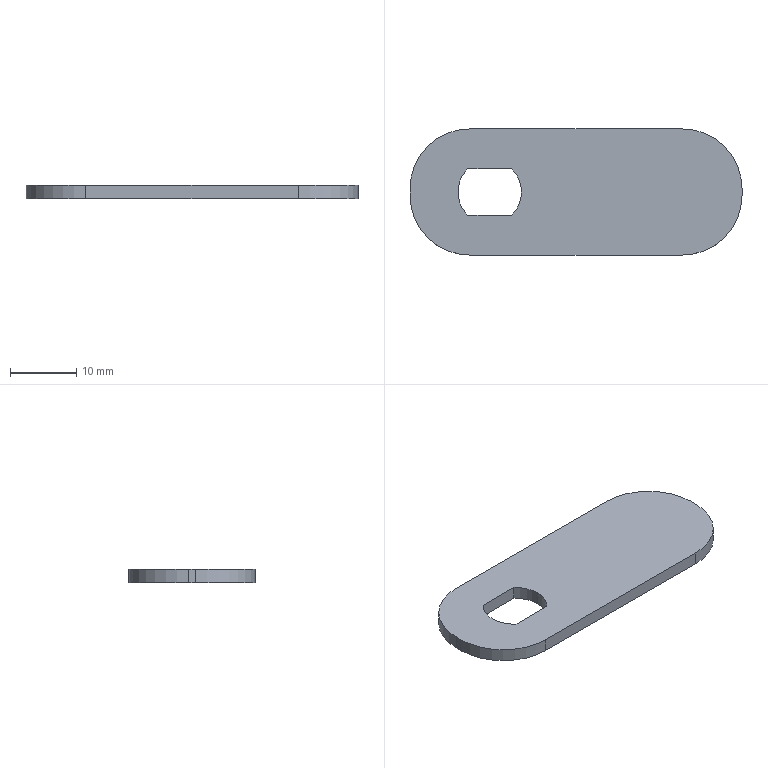Part | SolidWorks | features Fillet 1, FlatPattern 1, ICE 1, SMBaseFlange 1, SheetMetal 1 | 1 solid | 15 faces | box 50 x 19 x 2 mm | volume 1640 mm3 | plane 8 | cylinder 7 | commonest cylinder face diameters 18 x4 9.6 x3
STEP:
#1=CARTESIAN_POINT('',(-8.2,0.,-2.));
#2=VERTEX_POINT('',#1);
#3=CARTESIAN_POINT('',(-9.715,3.5,-2.));
#4=VERTEX_POINT('',#3);
#5=CARTESIAN_POINT('',(-13.,0.,-2.));
#6=DIRECTION('',(0.,0.,1.));
#7=DIRECTION('',(1.,0.,0.));
#8=AXIS2_PLACEMENT_3D('',#5,#6,#7);
#9=CIRCLE('',#8,4.8);
#10=EDGE_CURVE('',#2,#4,#9,.T.);
#11=ORIENTED_EDGE('',*,*,#10,.F.);
#12=CARTESIAN_POINT('',(-8.2,0.,0.));
#13=VERTEX_POINT('',#12);
#14=CARTESIAN_POINT('',(-8.2,0.,-10.));
#15=DIRECTION('',(0.,0.,1.));
#16=VECTOR('',#15,1000.);
#17=LINE('',#14,#16);
#18=EDGE_CURVE('',#2,#13,#17,.T.);
#19=ORIENTED_EDGE('',*,*,#18,.T.);
#20=CARTESIAN_POINT('',(-9.715,3.5,0.));
#21=VERTEX_POINT('',#20);
#22=CARTESIAN_POINT('',(-13.,0.,0.));
#23=DIRECTION('',(0.,0.,1.));
#24=DIRECTION('',(1.,0.,0.));
#25=AXIS2_PLACEMENT_3D('',#22,#23,#24);
#26=CIRCLE('',#25,4.8);
#27=EDGE_CURVE('',#13,#21,#26,.T.);
#28=ORIENTED_EDGE('',*,*,#27,.T.);
#29=CARTESIAN_POINT('',(-9.715,3.5,-10.));
#30=DIRECTION('',(0.,0.,1.));
#31=VECTOR('',#30,1000.);
#32=LINE('',#29,#31);
#33=EDGE_CURVE('',#4,#21,#32,.T.);
#34=ORIENTED_EDGE('',*,*,#33,.F.);
#35=EDGE_LOOP('',(#11,#19,#28,#34));
#36=FACE_OUTER_BOUND('',#35,.T.);
#37=CARTESIAN_POINT('',(-13.,0.,-10.));
#38=DIRECTION('',(0.,0.,1.));
#39=DIRECTION('',(1.,0.,0.));
#40=AXIS2_PLACEMENT_3D('',#37,#38,#39);
#41=CYLINDRICAL_SURFACE('',#40,4.8);
#42=ADVANCED_FACE('',(#36),#41,.F.);
#43=CARTESIAN_POINT('',(25.,-0.5,0.));
#44=VERTEX_POINT('',#43);
#45=CARTESIAN_POINT('',(25.,0.5,0.));
#46=VERTEX_POINT('',#45);
#47=CARTESIAN_POINT('',(25.,9.5,0.));
#48=DIRECTION('',(0.,1.,0.));
#49=VECTOR('',#48,1000.);
#50=LINE('',#47,#49);
#51=EDGE_CURVE('',#44,#46,#50,.T.);
#52=ORIENTED_EDGE('',*,*,#51,.F.);
#53=CARTESIAN_POINT('',(25.,-0.5,-2.));
#54=VERTEX_POINT('',#53);
#55=CARTESIAN_POINT('',(25.,-0.5,-2.));
#56=DIRECTION('',(0.,0.,-1.));
#57=VECTOR('',#56,1000.);
#58=LINE('',#55,#57);
#59=EDGE_CURVE('',#44,#54,#58,.T.);
#60=ORIENTED_EDGE('',*,*,#59,.T.);
#61=CARTESIAN_POINT('',(25.,0.5,-2.));
#62=VERTEX_POINT('',#61);
#63=CARTESIAN_POINT('',(25.,9.5,-2.));
#64=DIRECTION('',(0.,1.,0.));
#65=VECTOR('',#64,1000.);
#66=LINE('',#63,#65);
#67=EDGE_CURVE('',#54,#62,#66,.T.);
#68=ORIENTED_EDGE('',*,*,#67,.T.);
#69=CARTESIAN_POINT('',(25.,0.5,-2.));
#70=DIRECTION('',(0.,0.,1.));
#71=VECTOR('',#70,1000.);
#72=LINE('',#69,#71);
#73=EDGE_CURVE('',#62,#46,#72,.T.);
#74=ORIENTED_EDGE('',*,*,#73,.T.);
#75=EDGE_LOOP('',(#52,#60,#68,#74));
#76=FACE_OUTER_BOUND('',#75,.T.);
#77=CARTESIAN_POINT('',(25.,9.5,-2.));
#78=DIRECTION('',(1.,0.,0.));
#79=DIRECTION('',(0.,1.,0.));
#80=AXIS2_PLACEMENT_3D('',#77,#78,#79);
#81=PLANE('',#80);
#82=ADVANCED_FACE('',(#76),#81,.T.);
#83=CARTESIAN_POINT('',(-16.,-9.5,-2.));
#84=VERTEX_POINT('',#83);
#85=CARTESIAN_POINT('',(16.,-9.5,-2.));
#86=VERTEX_POINT('',#85);
#87=CARTESIAN_POINT('',(-25.,-9.5,-2.));
#88=DIRECTION('',(1.,0.,0.));
#89=VECTOR('',#88,1000.);
#90=LINE('',#87,#89);
#91=EDGE_CURVE('',#84,#86,#90,.T.);
#92=ORIENTED_EDGE('',*,*,#91,.T.);
#93=CARTESIAN_POINT('',(16.,-9.5,0.));
#94=VERTEX_POINT('',#93);
#95=CARTESIAN_POINT('',(16.,-9.5,-2.));
#96=DIRECTION('',(0.,0.,1.));
#97=VECTOR('',#96,1000.);
#98=LINE('',#95,#97);
#99=EDGE_CURVE('',#86,#94,#98,.T.);
#100=ORIENTED_EDGE('',*,*,#99,.T.);
#101=CARTESIAN_POINT('',(-16.,-9.5,0.));
#102=VERTEX_POINT('',#101);
#103=CARTESIAN_POINT('',(-25.,-9.5,0.));
#104=DIRECTION('',(1.,0.,0.));
#105=VECTOR('',#104,1000.);
#106=LINE('',#103,#105);
#107=EDGE_CURVE('',#102,#94,#106,.T.);
#108=ORIENTED_EDGE('',*,*,#107,.F.);
#109=CARTESIAN_POINT('',(-16.,-9.5,-2.));
#110=DIRECTION('',(0.,0.,-1.));
#111=VECTOR('',#110,1000.);
#112=LINE('',#109,#111);
#113=EDGE_CURVE('',#102,#84,#112,.T.);
#114=ORIENTED_EDGE('',*,*,#113,.T.);
#115=EDGE_LOOP('',(#92,#100,#108,#114));
#116=FACE_OUTER_BOUND('',#115,.T.);
#117=CARTESIAN_POINT('',(-25.,-9.5,-2.));
#118=DIRECTION('',(0.,-1.,0.));
#119=DIRECTION('',(0.,0.,-1.));
#120=AXIS2_PLACEMENT_3D('',#117,#118,#119);
#121=PLANE('',#120);
#122=ADVANCED_FACE('',(#116),#121,.T.);
#123=CARTESIAN_POINT('',(-25.,0.5,-2.));
#124=VERTEX_POINT('',#123);
#125=CARTESIAN_POINT('',(-25.,-0.5,-2.));
#126=VERTEX_POINT('',#125);
#127=CARTESIAN_POINT('',(-25.,9.5,-2.));
#128=DIRECTION('',(0.,-1.,0.));
#129=VECTOR('',#128,1000.);
#130=LINE('',#127,#129);
#131=EDGE_CURVE('',#124,#126,#130,.T.);
#132=ORIENTED_EDGE('',*,*,#131,.T.);
#133=CARTESIAN_POINT('',(-25.,-0.5,0.));
#134=VERTEX_POINT('',#133);
#135=CARTESIAN_POINT('',(-25.,-0.5,-2.));
#136=DIRECTION('',(0.,0.,1.));
#137=VECTOR('',#136,1000.);
#138=LINE('',#135,#137);
#139=EDGE_CURVE('',#126,#134,#138,.T.);
#140=ORIENTED_EDGE('',*,*,#139,.T.);
#141=CARTESIAN_POINT('',(-25.,0.5,0.));
#142=VERTEX_POINT('',#141);
#143=CARTESIAN_POINT('',(-25.,9.5,0.));
#144=DIRECTION('',(0.,-1.,0.));
#145=VECTOR('',#144,1000.);
#146=LINE('',#143,#145);
#147=EDGE_CURVE('',#142,#134,#146,.T.);
#148=ORIENTED_EDGE('',*,*,#147,.F.);
#149=CARTESIAN_POINT('',(-25.,0.5,-2.));
#150=DIRECTION('',(0.,0.,-1.));
#151=VECTOR('',#150,1000.);
#152=LINE('',#149,#151);
#153=EDGE_CURVE('',#142,#124,#152,.T.);
#154=ORIENTED_EDGE('',*,*,#153,.T.);
#155=EDGE_LOOP('',(#132,#140,#148,#154));
#156=FACE_OUTER_BOUND('',#155,.T.);
#157=CARTESIAN_POINT('',(-25.,9.5,-2.));
#158=DIRECTION('',(-1.,0.,0.));
#159=DIRECTION('',(0.,0.,1.));
#160=AXIS2_PLACEMENT_3D('',#157,#158,#159);
#161=PLANE('',#160);
#162=ADVANCED_FACE('',(#156),#161,.T.);
#163=CARTESIAN_POINT('',(16.,9.5,0.));
#164=VERTEX_POINT('',#163);
#165=CARTESIAN_POINT('',(-16.,9.5,0.));
#166=VERTEX_POINT('',#165);
#167=CARTESIAN_POINT('',(-25.,9.5,0.));
#168=DIRECTION('',(-1.,0.,0.));
#169=VECTOR('',#168,1000.);
#170=LINE('',#167,#169);
#171=EDGE_CURVE('',#164,#166,#170,.T.);
#172=ORIENTED_EDGE('',*,*,#171,.F.);
#173=CARTESIAN_POINT('',(16.,9.5,-2.));
#174=VERTEX_POINT('',#173);
#175=CARTESIAN_POINT('',(16.,9.5,-2.));
#176=DIRECTION('',(0.,0.,-1.));
#177=VECTOR('',#176,1000.);
#178=LINE('',#175,#177);
#179=EDGE_CURVE('',#164,#174,#178,.T.);
#180=ORIENTED_EDGE('',*,*,#179,.T.);
#181=CARTESIAN_POINT('',(-16.,9.5,-2.));
#182=VERTEX_POINT('',#181);
#183=CARTESIAN_POINT('',(-25.,9.5,-2.));
#184=DIRECTION('',(-1.,0.,0.));
#185=VECTOR('',#184,1000.);
#186=LINE('',#183,#185);
#187=EDGE_CURVE('',#174,#182,#186,.T.);
#188=ORIENTED_EDGE('',*,*,#187,.T.);
#189=CARTESIAN_POINT('',(-16.,9.5,-2.));
#190=DIRECTION('',(0.,0.,1.));
#191=VECTOR('',#190,1000.);
#192=LINE('',#189,#191);
#193=EDGE_CURVE('',#182,#166,#192,.T.);
#194=ORIENTED_EDGE('',*,*,#193,.T.);
#195=EDGE_LOOP('',(#172,#180,#188,#194));
#196=FACE_OUTER_BOUND('',#195,.T.);
#197=CARTESIAN_POINT('',(-25.,9.5,-2.));
#198=DIRECTION('',(0.,1.,0.));
#199=DIRECTION('',(0.,0.,1.));
#200=AXIS2_PLACEMENT_3D('',#197,#198,#199);
#201=PLANE('',#200);
#202=ADVANCED_FACE('',(#196),#201,.T.);
#203=CARTESIAN_POINT('',(-16.285,-3.5,-2.));
#204=VERTEX_POINT('',#203);
#205=CARTESIAN_POINT('',(-9.715,-3.5,-2.));
#206=VERTEX_POINT('',#205);
#207=CARTESIAN_POINT('',(0.,-3.5,-2.));
#208=DIRECTION('',(1.,0.,0.));
#209=VECTOR('',#208,1000.);
#210=LINE('',#207,#209);
#211=EDGE_CURVE('',#204,#206,#210,.T.);
#212=ORIENTED_EDGE('',*,*,#211,.T.);
#213=CARTESIAN_POINT('',(-13.,0.,-2.));
#214=DIRECTION('',(0.,0.,1.));
#215=DIRECTION('',(1.,0.,0.));
#216=AXIS2_PLACEMENT_3D('',#213,#214,#215);
#217=CIRCLE('',#216,4.8);
#218=EDGE_CURVE('',#206,#2,#217,.T.);
#219=ORIENTED_EDGE('',*,*,#218,.T.);
#220=ORIENTED_EDGE('',*,*,#10,.T.);
#221=CARTESIAN_POINT('',(-16.285,3.5,-2.));
#222=VERTEX_POINT('',#221);
#223=CARTESIAN_POINT('',(0.,3.5,-2.));
#224=DIRECTION('',(-1.,0.,0.));
#225=VECTOR('',#224,1000.);
#226=LINE('',#223,#225);
#227=EDGE_CURVE('',#4,#222,#226,.T.);
#228=ORIENTED_EDGE('',*,*,#227,.T.);
#229=CARTESIAN_POINT('',(-13.,0.,-2.));
#230=DIRECTION('',(0.,0.,1.));
#231=DIRECTION('',(1.,0.,0.));
#232=AXIS2_PLACEMENT_3D('',#229,#230,#231);
#233=CIRCLE('',#232,4.8);
#234=EDGE_CURVE('',#222,#204,#233,.T.);
#235=ORIENTED_EDGE('',*,*,#234,.T.);
#236=EDGE_LOOP('',(#212,#219,#220,#228,#235));
#237=FACE_BOUND('',#236,.T.);
#238=ORIENTED_EDGE('',*,*,#67,.F.);
#239=CARTESIAN_POINT('',(16.,-0.5,-2.));
#240=DIRECTION('',(0.,0.,-1.));
#241=DIRECTION('',(1.,0.,0.));
#242=AXIS2_PLACEMENT_3D('',#239,#240,#241);
#243=CIRCLE('',#242,9.);
#244=EDGE_CURVE('',#54,#86,#243,.T.);
#245=ORIENTED_EDGE('',*,*,#244,.T.);
#246=ORIENTED_EDGE('',*,*,#91,.F.);
#247=CARTESIAN_POINT('',(-16.,-0.5,-2.));
#248=DIRECTION('',(0.,0.,-1.));
#249=DIRECTION('',(1.,0.,0.));
#250=AXIS2_PLACEMENT_3D('',#247,#248,#249);
#251=CIRCLE('',#250,9.);
#252=EDGE_CURVE('',#84,#126,#251,.T.);
#253=ORIENTED_EDGE('',*,*,#252,.T.);
#254=ORIENTED_EDGE('',*,*,#131,.F.);
#255=CARTESIAN_POINT('',(-16.,0.5,-2.));
#256=DIRECTION('',(0.,0.,-1.));
#257=DIRECTION('',(1.,0.,0.));
#258=AXIS2_PLACEMENT_3D('',#255,#256,#257);
#259=CIRCLE('',#258,9.);
#260=EDGE_CURVE('',#124,#182,#259,.T.);
#261=ORIENTED_EDGE('',*,*,#260,.T.);
#262=ORIENTED_EDGE('',*,*,#187,.F.);
#263=CARTESIAN_POINT('',(16.,0.5,-2.));
#264=DIRECTION('',(0.,0.,-1.));
#265=DIRECTION('',(1.,0.,0.));
#266=AXIS2_PLACEMENT_3D('',#263,#264,#265);
#267=CIRCLE('',#266,9.);
#268=EDGE_CURVE('',#174,#62,#267,.T.);
#269=ORIENTED_EDGE('',*,*,#268,.T.);
#270=EDGE_LOOP('',(#238,#245,#246,#253,#254,#261,#262,#269));
#271=FACE_OUTER_BOUND('',#270,.T.);
#272=CARTESIAN_POINT('',(0.,0.,-2.));
#273=DIRECTION('',(0.,0.,1.));
#274=DIRECTION('',(1.,0.,0.));
#275=AXIS2_PLACEMENT_3D('',#272,#273,#274);
#276=PLANE('',#275);
#277=ADVANCED_FACE('',(#237,#271),#276,.F.);
#278=CARTESIAN_POINT('',(-9.715,-3.5,0.));
#279=VERTEX_POINT('',#278);
#280=CARTESIAN_POINT('',(-13.,0.,0.));
#281=DIRECTION('',(0.,0.,1.));
#282=DIRECTION('',(1.,0.,0.));
#283=AXIS2_PLACEMENT_3D('',#280,#281,#282);
#284=CIRCLE('',#283,4.8);
#285=EDGE_CURVE('',#279,#13,#284,.T.);
#286=ORIENTED_EDGE('',*,*,#285,.F.);
#287=CARTESIAN_POINT('',(-16.285,-3.5,0.));
#288=VERTEX_POINT('',#287);
#289=CARTESIAN_POINT('',(-16.285,-3.5,0.));
#290=DIRECTION('',(1.,0.,0.));
#291=VECTOR('',#290,1000.);
#292=LINE('',#289,#291);
#293=EDGE_CURVE('',#288,#279,#292,.T.);
#294=ORIENTED_EDGE('',*,*,#293,.F.);
#295=CARTESIAN_POINT('',(-16.285,3.5,0.));
#296=VERTEX_POINT('',#295);
#297=CARTESIAN_POINT('',(-13.,0.,0.));
#298=DIRECTION('',(0.,0.,1.));
#299=DIRECTION('',(1.,0.,0.));
#300=AXIS2_PLACEMENT_3D('',#297,#298,#299);
#301=CIRCLE('',#300,4.8);
#302=EDGE_CURVE('',#296,#288,#301,.T.);
#303=ORIENTED_EDGE('',*,*,#302,.F.);
#304=CARTESIAN_POINT('',(-16.285,3.5,0.));
#305=DIRECTION('',(-1.,0.,0.));
#306=VECTOR('',#305,1000.);
#307=LINE('',#304,#306);
#308=EDGE_CURVE('',#21,#296,#307,.T.);
#309=ORIENTED_EDGE('',*,*,#308,.F.);
#310=ORIENTED_EDGE('',*,*,#27,.F.);
#311=EDGE_LOOP('',(#286,#294,#303,#309,#310));
#312=FACE_BOUND('',#311,.T.);
#313=ORIENTED_EDGE('',*,*,#107,.T.);
#314=CARTESIAN_POINT('',(16.,-0.5,0.));
#315=DIRECTION('',(0.,0.,1.));
#316=DIRECTION('',(1.,0.,0.));
#317=AXIS2_PLACEMENT_3D('',#314,#315,#316);
#318=CIRCLE('',#317,9.);
#319=EDGE_CURVE('',#94,#44,#318,.T.);
#320=ORIENTED_EDGE('',*,*,#319,.T.);
#321=ORIENTED_EDGE('',*,*,#51,.T.);
#322=CARTESIAN_POINT('',(16.,0.5,0.));
#323=DIRECTION('',(0.,0.,1.));
#324=DIRECTION('',(1.,0.,0.));
#325=AXIS2_PLACEMENT_3D('',#322,#323,#324);
#326=CIRCLE('',#325,9.);
#327=EDGE_CURVE('',#46,#164,#326,.T.);
#328=ORIENTED_EDGE('',*,*,#327,.T.);
#329=ORIENTED_EDGE('',*,*,#171,.T.);
#330=CARTESIAN_POINT('',(-16.,0.5,0.));
#331=DIRECTION('',(0.,0.,1.));
#332=DIRECTION('',(1.,0.,0.));
#333=AXIS2_PLACEMENT_3D('',#330,#331,#332);
#334=CIRCLE('',#333,9.);
#335=EDGE_CURVE('',#166,#142,#334,.T.);
#336=ORIENTED_EDGE('',*,*,#335,.T.);
#337=ORIENTED_EDGE('',*,*,#147,.T.);
#338=CARTESIAN_POINT('',(-16.,-0.5,0.));
#339=DIRECTION('',(0.,0.,1.));
#340=DIRECTION('',(1.,0.,0.));
#341=AXIS2_PLACEMENT_3D('',#338,#339,#340);
#342=CIRCLE('',#341,9.);
#343=EDGE_CURVE('',#134,#102,#342,.T.);
#344=ORIENTED_EDGE('',*,*,#343,.T.);
#345=EDGE_LOOP('',(#313,#320,#321,#328,#329,#336,#337,#344));
#346=FACE_OUTER_BOUND('',#345,.T.);
#347=CARTESIAN_POINT('',(0.,0.,0.));
#348=DIRECTION('',(0.,0.,1.));
#349=DIRECTION('',(1.,0.,0.));
#350=AXIS2_PLACEMENT_3D('',#347,#348,#349);
#351=PLANE('',#350);
#352=ADVANCED_FACE('',(#312,#346),#351,.T.);
#353=ORIENTED_EDGE('',*,*,#18,.F.);
#354=ORIENTED_EDGE('',*,*,#218,.F.);
#355=CARTESIAN_POINT('',(-9.715,-3.5,-10.));
#356=DIRECTION('',(0.,0.,1.));
#357=VECTOR('',#356,1000.);
#358=LINE('',#355,#357);
#359=EDGE_CURVE('',#206,#279,#358,.T.);
#360=ORIENTED_EDGE('',*,*,#359,.T.);
#361=ORIENTED_EDGE('',*,*,#285,.T.);
#362=EDGE_LOOP('',(#353,#354,#360,#361));
#363=FACE_OUTER_BOUND('',#362,.T.);
#364=CARTESIAN_POINT('',(-13.,0.,-10.));
#365=DIRECTION('',(0.,0.,1.));
#366=DIRECTION('',(1.,0.,0.));
#367=AXIS2_PLACEMENT_3D('',#364,#365,#366);
#368=CYLINDRICAL_SURFACE('',#367,4.8);
#369=ADVANCED_FACE('',(#363),#368,.F.);
#370=CARTESIAN_POINT('',(-16.285,-3.5,-10.));
#371=DIRECTION('',(0.,0.,1.));
#372=VECTOR('',#371,1000.);
#373=LINE('',#370,#372);
#374=EDGE_CURVE('',#204,#288,#373,.T.);
#375=ORIENTED_EDGE('',*,*,#374,.T.);
#376=ORIENTED_EDGE('',*,*,#293,.T.);
#377=ORIENTED_EDGE('',*,*,#359,.F.);
#378=ORIENTED_EDGE('',*,*,#211,.F.);
#379=EDGE_LOOP('',(#375,#376,#377,#378));
#380=FACE_OUTER_BOUND('',#379,.T.);
#381=CARTESIAN_POINT('',(-16.285,-3.5,-10.));
#382=DIRECTION('',(0.,-1.,0.));
#383=DIRECTION('',(0.,0.,-1.));
#384=AXIS2_PLACEMENT_3D('',#381,#382,#383);
#385=PLANE('',#384);
#386=ADVANCED_FACE('',(#380),#385,.F.);
#387=CARTESIAN_POINT('',(-16.285,3.5,-10.));
#388=DIRECTION('',(0.,0.,1.));
#389=VECTOR('',#388,1000.);
#390=LINE('',#387,#389);
#391=EDGE_CURVE('',#222,#296,#390,.T.);
#392=ORIENTED_EDGE('',*,*,#391,.T.);
#393=ORIENTED_EDGE('',*,*,#302,.T.);
#394=ORIENTED_EDGE('',*,*,#374,.F.);
#395=ORIENTED_EDGE('',*,*,#234,.F.);
#396=EDGE_LOOP('',(#392,#393,#394,#395));
#397=FACE_OUTER_BOUND('',#396,.T.);
#398=CARTESIAN_POINT('',(-13.,0.,-10.));
#399=DIRECTION('',(0.,0.,1.));
#400=DIRECTION('',(1.,0.,0.));
#401=AXIS2_PLACEMENT_3D('',#398,#399,#400);
#402=CYLINDRICAL_SURFACE('',#401,4.8);
#403=ADVANCED_FACE('',(#397),#402,.F.);
#404=ORIENTED_EDGE('',*,*,#33,.T.);
#405=ORIENTED_EDGE('',*,*,#308,.T.);
#406=ORIENTED_EDGE('',*,*,#391,.F.);
#407=ORIENTED_EDGE('',*,*,#227,.F.);
#408=EDGE_LOOP('',(#404,#405,#406,#407));
#409=FACE_OUTER_BOUND('',#408,.T.);
#410=CARTESIAN_POINT('',(-16.285,3.5,-10.));
#411=DIRECTION('',(0.,1.,0.));
#412=DIRECTION('',(0.,0.,1.));
#413=AXIS2_PLACEMENT_3D('',#410,#411,#412);
#414=PLANE('',#413);
#415=ADVANCED_FACE('',(#409),#414,.F.);
#416=ORIENTED_EDGE('',*,*,#244,.F.);
#417=ORIENTED_EDGE('',*,*,#59,.F.);
#418=ORIENTED_EDGE('',*,*,#319,.F.);
#419=ORIENTED_EDGE('',*,*,#99,.F.);
#420=EDGE_LOOP('',(#416,#417,#418,#419));
#421=FACE_OUTER_BOUND('',#420,.T.);
#422=CARTESIAN_POINT('',(16.,-0.5,-2.));
#423=DIRECTION('',(0.,0.,1.));
#424=DIRECTION('',(1.,0.,0.));
#425=AXIS2_PLACEMENT_3D('',#422,#423,#424);
#426=CYLINDRICAL_SURFACE('',#425,9.);
#427=ADVANCED_FACE('',(#421),#426,.T.);
#428=ORIENTED_EDGE('',*,*,#268,.F.);
#429=ORIENTED_EDGE('',*,*,#179,.F.);
#430=ORIENTED_EDGE('',*,*,#327,.F.);
#431=ORIENTED_EDGE('',*,*,#73,.F.);
#432=EDGE_LOOP('',(#428,#429,#430,#431));
#433=FACE_OUTER_BOUND('',#432,.T.);
#434=CARTESIAN_POINT('',(16.,0.5,-2.));
#435=DIRECTION('',(0.,0.,1.));
#436=DIRECTION('',(1.,0.,0.));
#437=AXIS2_PLACEMENT_3D('',#434,#435,#436);
#438=CYLINDRICAL_SURFACE('',#437,9.);
#439=ADVANCED_FACE('',(#433),#438,.T.);
#440=ORIENTED_EDGE('',*,*,#252,.F.);
#441=ORIENTED_EDGE('',*,*,#113,.F.);
#442=ORIENTED_EDGE('',*,*,#343,.F.);
#443=ORIENTED_EDGE('',*,*,#139,.F.);
#444=EDGE_LOOP('',(#440,#441,#442,#443));
#445=FACE_OUTER_BOUND('',#444,.T.);
#446=CARTESIAN_POINT('',(-16.,-0.5,-2.));
#447=DIRECTION('',(0.,0.,1.));
#448=DIRECTION('',(1.,0.,0.));
#449=AXIS2_PLACEMENT_3D('',#446,#447,#448);
#450=CYLINDRICAL_SURFACE('',#449,9.);
#451=ADVANCED_FACE('',(#445),#450,.T.);
#452=ORIENTED_EDGE('',*,*,#260,.F.);
#453=ORIENTED_EDGE('',*,*,#153,.F.);
#454=ORIENTED_EDGE('',*,*,#335,.F.);
#455=ORIENTED_EDGE('',*,*,#193,.F.);
#456=EDGE_LOOP('',(#452,#453,#454,#455));
#457=FACE_OUTER_BOUND('',#456,.T.);
#458=CARTESIAN_POINT('',(-16.,0.5,-2.));
#459=DIRECTION('',(0.,0.,1.));
#460=DIRECTION('',(1.,0.,0.));
#461=AXIS2_PLACEMENT_3D('',#458,#459,#460);
#462=CYLINDRICAL_SURFACE('',#461,9.);
#463=ADVANCED_FACE('',(#457),#462,.T.);
#464=CLOSED_SHELL('',(#42,#82,#122,#162,#202,#277,#352,#369,#386,#403,#415,#427,#439,#451,#463));
#465=MANIFOLD_SOLID_BREP('',#464);
#466=CARTESIAN_POINT('',(0.,0.,0.));
#467=DIRECTION('',(0.,0.,1.));
#468=DIRECTION('',(1.,0.,0.));
#469=AXIS2_PLACEMENT_3D('',#466,#467,#468);
#470=(LENGTH_UNIT()NAMED_UNIT(*)SI_UNIT(.MILLI.,.METRE.));
#471=UNCERTAINTY_MEASURE_WITH_UNIT(LENGTH_MEASURE(0.00001),#470,'','');
#472=(NAMED_UNIT(*)PLANE_ANGLE_UNIT()SI_UNIT($,.RADIAN.));
#473=(NAMED_UNIT(*)SI_UNIT($,.STERADIAN.)SOLID_ANGLE_UNIT());
#474=(GEOMETRIC_REPRESENTATION_CONTEXT(3)GLOBAL_UNCERTAINTY_ASSIGNED_CONTEXT((#471))GLOBAL_UNIT_ASSIGNED_CONTEXT((#470,#472,#473))REPRESENTATION_CONTEXT('',''));
#475=ADVANCED_BREP_SHAPE_REPRESENTATION('',(#465,#469),#474);